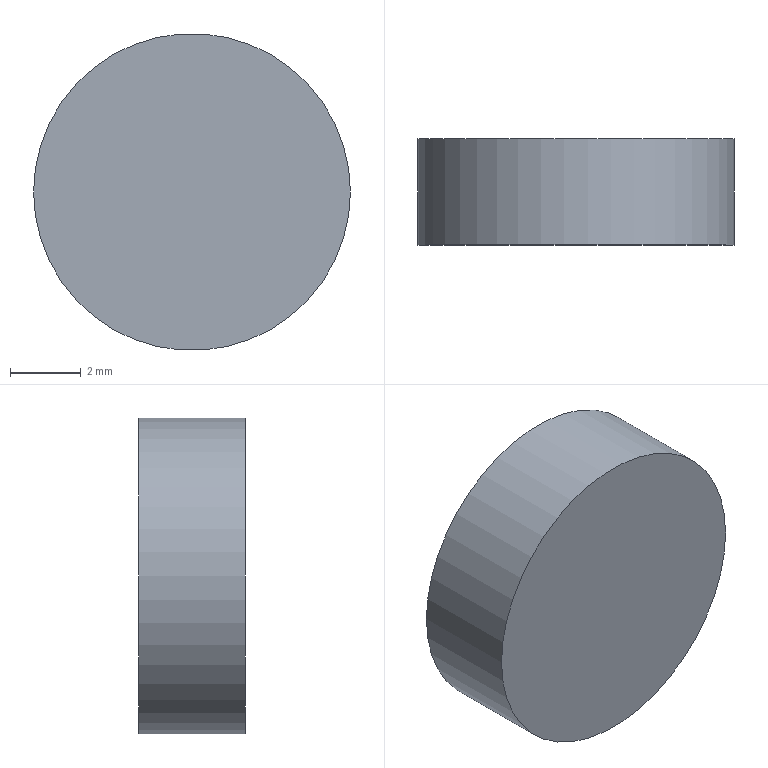Part | STEP file | 1_id286_x_t | 1 solid | 3 faces | box 8.95 x 3 x 8.95 mm | volume 188.737 mm3 | plane 2 | cylinder 1 | commonest cylinder face diameters 8.95 x1
STEP:
#1=CARTESIAN_POINT('',(0.,0.,0.));
#2=DIRECTION('',(0.,0.,1.));
#3=DIRECTION('',(1.,0.,0.));
#4=AXIS2_PLACEMENT_3D('',#1,#2,#3);
#5=CARTESIAN_POINT('',(730.25,175.025,-70.67));
#6=VERTEX_POINT('',#5);
#7=CARTESIAN_POINT('',(739.2,175.025,-70.67));
#8=VERTEX_POINT('',#7);
#9=CARTESIAN_POINT('',(734.725,175.025,-70.67));
#10=DIRECTION('',(0.,-1.,0.));
#11=DIRECTION('',(-1.,0.,0.));
#12=AXIS2_PLACEMENT_3D('',#9,#10,#11);
#13=CIRCLE('',#12,4.475);
#14=CARTESIAN_POINT('',(734.725,172.025,-70.67));
#15=DIRECTION('',(0.,1.,0.));
#16=DIRECTION('',(0.,0.,1.));
#17=AXIS2_PLACEMENT_3D('',#14,#15,#16);
#18=CYLINDRICAL_SURFACE('',#17,4.475);
#19=CARTESIAN_POINT('',(4.712,3.));
#20=DIRECTION('',(-1.,0.));
#21=VECTOR('',#20,1.);
#22=LINE('',#19,#21);
#23=(GEOMETRIC_REPRESENTATION_CONTEXT(2)PARAMETRIC_REPRESENTATION_CONTEXT()REPRESENTATION_CONTEXT('',''));
#24=DEFINITIONAL_REPRESENTATION('',(#22),#23);
#25=PCURVE('',#18,#24);
#26=CARTESIAN_POINT('',(734.725,175.025,-70.67));
#27=DIRECTION('',(0.,-1.,0.));
#28=DIRECTION('',(0.,0.,-1.));
#29=AXIS2_PLACEMENT_3D('',#26,#27,#28);
#30=PLANE('',#29);
#31=CARTESIAN_POINT('',(0.,0.));
#32=DIRECTION('',(0.,-1.));
#33=AXIS2_PLACEMENT_2D('',#31,#32);
#34=CIRCLE('',#33,4.475);
#35=(GEOMETRIC_REPRESENTATION_CONTEXT(2)PARAMETRIC_REPRESENTATION_CONTEXT()REPRESENTATION_CONTEXT('',''));
#36=DEFINITIONAL_REPRESENTATION('',(#34),#35);
#37=PCURVE('',#30,#36);
#38=SURFACE_CURVE('',#13,(#25,#37),.PCURVE_S1.);
#39=EDGE_CURVE('',#6,#8,#38,.T.);
#40=ORIENTED_EDGE('',*,*,#39,.T.);
#41=CARTESIAN_POINT('',(739.2,172.025,-70.67));
#42=VERTEX_POINT('',#41);
#43=CARTESIAN_POINT('',(739.2,172.025,-70.67));
#44=CARTESIAN_POINT('',(739.2,175.025,-70.67));
#45=B_SPLINE_CURVE_WITH_KNOTS('',1,(#43,#44),.UNSPECIFIED.,.F.,.F.,(2,2),(0.,3.),.PIECEWISE_BEZIER_KNOTS.);
#46=CARTESIAN_POINT('',(1.571,0.));
#47=DIRECTION('',(0.,1.));
#48=VECTOR('',#47,1.);
#49=LINE('',#46,#48);
#50=(GEOMETRIC_REPRESENTATION_CONTEXT(2)PARAMETRIC_REPRESENTATION_CONTEXT()REPRESENTATION_CONTEXT('',''));
#51=DEFINITIONAL_REPRESENTATION('',(#49),#50);
#52=PCURVE('',#18,#51);
#53=CARTESIAN_POINT('',(7.854,0.));
#54=DIRECTION('',(0.,1.));
#55=VECTOR('',#54,1.);
#56=LINE('',#53,#55);
#57=(GEOMETRIC_REPRESENTATION_CONTEXT(2)PARAMETRIC_REPRESENTATION_CONTEXT()REPRESENTATION_CONTEXT('',''));
#58=DEFINITIONAL_REPRESENTATION('',(#56),#57);
#59=PCURVE('',#18,#58);
#60=SEAM_CURVE('',#45,(#52,#59),.PCURVE_S1.);
#61=EDGE_CURVE('',#42,#8,#60,.T.);
#62=ORIENTED_EDGE('',*,*,#61,.F.);
#63=CARTESIAN_POINT('',(734.725,172.025,-70.67));
#64=DIRECTION('',(0.,-1.,0.));
#65=DIRECTION('',(1.,0.,0.));
#66=AXIS2_PLACEMENT_3D('',#63,#64,#65);
#67=CIRCLE('',#66,4.475);
#68=CARTESIAN_POINT('',(7.854,0.));
#69=DIRECTION('',(-1.,0.));
#70=VECTOR('',#69,1.);
#71=LINE('',#68,#70);
#72=(GEOMETRIC_REPRESENTATION_CONTEXT(2)PARAMETRIC_REPRESENTATION_CONTEXT()REPRESENTATION_CONTEXT('',''));
#73=DEFINITIONAL_REPRESENTATION('',(#71),#72);
#74=PCURVE('',#18,#73);
#75=CARTESIAN_POINT('',(734.725,172.025,-70.67));
#76=DIRECTION('',(0.,-1.,0.));
#77=DIRECTION('',(0.,0.,-1.));
#78=AXIS2_PLACEMENT_3D('',#75,#76,#77);
#79=PLANE('',#78);
#80=CARTESIAN_POINT('',(0.,0.));
#81=DIRECTION('',(0.,1.));
#82=AXIS2_PLACEMENT_2D('',#80,#81);
#83=CIRCLE('',#82,4.475);
#84=(GEOMETRIC_REPRESENTATION_CONTEXT(2)PARAMETRIC_REPRESENTATION_CONTEXT()REPRESENTATION_CONTEXT('',''));
#85=DEFINITIONAL_REPRESENTATION('',(#83),#84);
#86=PCURVE('',#79,#85);
#87=SURFACE_CURVE('',#67,(#74,#86),.PCURVE_S1.);
#88=EDGE_CURVE('',#42,#42,#87,.T.);
#89=ORIENTED_EDGE('',*,*,#88,.F.);
#90=ORIENTED_EDGE('',*,*,#61,.T.);
#91=CARTESIAN_POINT('',(734.725,175.025,-70.67));
#92=DIRECTION('',(0.,-1.,0.));
#93=DIRECTION('',(-1.,0.,0.));
#94=AXIS2_PLACEMENT_3D('',#91,#92,#93);
#95=CIRCLE('',#94,4.475);
#96=CARTESIAN_POINT('',(10.996,3.));
#97=DIRECTION('',(-1.,0.));
#98=VECTOR('',#97,1.);
#99=LINE('',#96,#98);
#100=(GEOMETRIC_REPRESENTATION_CONTEXT(2)PARAMETRIC_REPRESENTATION_CONTEXT()REPRESENTATION_CONTEXT('',''));
#101=DEFINITIONAL_REPRESENTATION('',(#99),#100);
#102=PCURVE('',#18,#101);
#103=CARTESIAN_POINT('',(0.,0.));
#104=DIRECTION('',(0.,-1.));
#105=AXIS2_PLACEMENT_2D('',#103,#104);
#106=CIRCLE('',#105,4.475);
#107=(GEOMETRIC_REPRESENTATION_CONTEXT(2)PARAMETRIC_REPRESENTATION_CONTEXT()REPRESENTATION_CONTEXT('',''));
#108=DEFINITIONAL_REPRESENTATION('',(#106),#107);
#109=PCURVE('',#30,#108);
#110=SURFACE_CURVE('',#95,(#102,#109),.PCURVE_S1.);
#111=EDGE_CURVE('',#8,#6,#110,.T.);
#112=ORIENTED_EDGE('',*,*,#111,.T.);
#113=EDGE_LOOP('',(#40,#62,#89,#90,#112));
#114=FACE_BOUND('',#113,.T.);
#115=ADVANCED_FACE('',(#114),#18,.T.);
#116=ORIENTED_EDGE('',*,*,#88,.T.);
#117=EDGE_LOOP('',(#116));
#118=FACE_BOUND('',#117,.T.);
#119=ADVANCED_FACE('',(#118),#79,.T.);
#120=ORIENTED_EDGE('',*,*,#39,.F.);
#121=ORIENTED_EDGE('',*,*,#111,.F.);
#122=EDGE_LOOP('',(#120,#121));
#123=FACE_BOUND('',#122,.T.);
#124=ADVANCED_FACE('',(#123),#30,.F.);
#125=CLOSED_SHELL('',(#115,#119,#124));
#126=MANIFOLD_SOLID_BREP('',#125);
#127=(LENGTH_UNIT()NAMED_UNIT(*)SI_UNIT(.MILLI.,.METRE.));
#128=UNCERTAINTY_MEASURE_WITH_UNIT(LENGTH_MEASURE(0.000005),#127,'','');
#129=(NAMED_UNIT(*)PLANE_ANGLE_UNIT()SI_UNIT($,.RADIAN.));
#130=(NAMED_UNIT(*)SI_UNIT($,.STERADIAN.)SOLID_ANGLE_UNIT());
#131=(GEOMETRIC_REPRESENTATION_CONTEXT(3)GLOBAL_UNCERTAINTY_ASSIGNED_CONTEXT((#128))GLOBAL_UNIT_ASSIGNED_CONTEXT((#127,#129,#130))REPRESENTATION_CONTEXT('',''));
#132=ADVANCED_BREP_SHAPE_REPRESENTATION('',(#4,#126),#131);